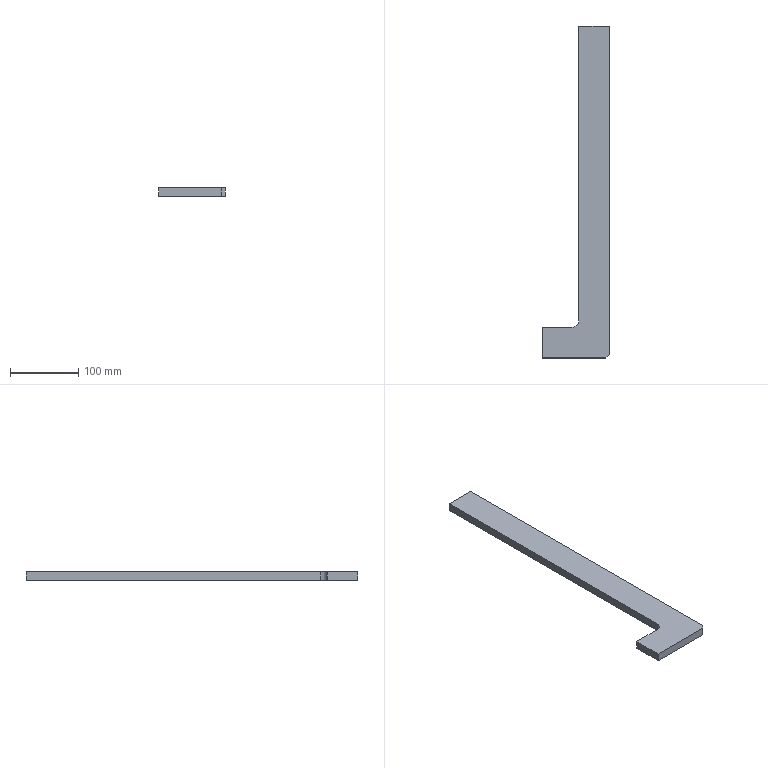Part | SolidWorks | features Chamfer 1, Extrusion 1, Fillet 1, ICE 1 | 1 solid | 10 faces | box 98 x 488 x 12 mm | volume 292248 mm3 | plane 9 | cylinder 1 | commonest cylinder face diameters 20 x1
STEP:
#1=CARTESIAN_POINT('',(49.,-239.,6.));
#2=VERTEX_POINT('',#1);
#3=CARTESIAN_POINT('',(49.,244.,6.));
#4=VERTEX_POINT('',#3);
#5=CARTESIAN_POINT('',(49.,-244.,6.));
#6=DIRECTION('',(0.,1.,0.));
#7=VECTOR('',#6,1000.);
#8=LINE('',#5,#7);
#9=EDGE_CURVE('',#2,#4,#8,.T.);
#10=ORIENTED_EDGE('',*,*,#9,.F.);
#11=CARTESIAN_POINT('',(49.,-239.,-6.));
#12=VERTEX_POINT('',#11);
#13=CARTESIAN_POINT('',(49.,-239.,6.));
#14=DIRECTION('',(0.,0.,-1.));
#15=VECTOR('',#14,1000.);
#16=LINE('',#13,#15);
#17=EDGE_CURVE('',#2,#12,#16,.T.);
#18=ORIENTED_EDGE('',*,*,#17,.T.);
#19=CARTESIAN_POINT('',(49.,244.,-6.));
#20=VERTEX_POINT('',#19);
#21=CARTESIAN_POINT('',(49.,-244.,-6.));
#22=DIRECTION('',(0.,1.,0.));
#23=VECTOR('',#22,1000.);
#24=LINE('',#21,#23);
#25=EDGE_CURVE('',#12,#20,#24,.T.);
#26=ORIENTED_EDGE('',*,*,#25,.T.);
#27=CARTESIAN_POINT('',(49.,244.,6.));
#28=DIRECTION('',(0.,0.,-1.));
#29=VECTOR('',#28,1000.);
#30=LINE('',#27,#29);
#31=EDGE_CURVE('',#4,#20,#30,.T.);
#32=ORIENTED_EDGE('',*,*,#31,.F.);
#33=EDGE_LOOP('',(#10,#18,#26,#32));
#34=FACE_OUTER_BOUND('',#33,.T.);
#35=CARTESIAN_POINT('',(49.,-244.,6.));
#36=DIRECTION('',(-1.,0.,0.));
#37=DIRECTION('',(0.,0.,1.));
#38=AXIS2_PLACEMENT_3D('',#35,#36,#37);
#39=PLANE('',#38);
#40=ADVANCED_FACE('',(#34),#39,.F.);
#41=CARTESIAN_POINT('',(4.,244.,-6.));
#42=VERTEX_POINT('',#41);
#43=CARTESIAN_POINT('',(-49.,244.,-6.));
#44=DIRECTION('',(-1.,0.,0.));
#45=VECTOR('',#44,1000.);
#46=LINE('',#43,#45);
#47=EDGE_CURVE('',#20,#42,#46,.T.);
#48=ORIENTED_EDGE('',*,*,#47,.T.);
#49=CARTESIAN_POINT('',(4.,244.,6.));
#50=VERTEX_POINT('',#49);
#51=CARTESIAN_POINT('',(4.,244.,-6.001));
#52=DIRECTION('',(0.,0.,1.));
#53=VECTOR('',#52,1000.);
#54=LINE('',#51,#53);
#55=EDGE_CURVE('',#42,#50,#54,.T.);
#56=ORIENTED_EDGE('',*,*,#55,.T.);
#57=CARTESIAN_POINT('',(-49.,244.,6.));
#58=DIRECTION('',(-1.,0.,0.));
#59=VECTOR('',#58,1000.);
#60=LINE('',#57,#59);
#61=EDGE_CURVE('',#4,#50,#60,.T.);
#62=ORIENTED_EDGE('',*,*,#61,.F.);
#63=ORIENTED_EDGE('',*,*,#31,.T.);
#64=EDGE_LOOP('',(#48,#56,#62,#63));
#65=FACE_OUTER_BOUND('',#64,.T.);
#66=CARTESIAN_POINT('',(-49.,244.,6.));
#67=DIRECTION('',(0.,-1.,0.));
#68=DIRECTION('',(0.,0.,-1.));
#69=AXIS2_PLACEMENT_3D('',#66,#67,#68);
#70=PLANE('',#69);
#71=ADVANCED_FACE('',(#65),#70,.F.);
#72=CARTESIAN_POINT('',(-49.,-199.,6.));
#73=VERTEX_POINT('',#72);
#74=CARTESIAN_POINT('',(-49.,-244.,6.));
#75=VERTEX_POINT('',#74);
#76=CARTESIAN_POINT('',(-49.,-244.,6.));
#77=DIRECTION('',(0.,-1.,0.));
#78=VECTOR('',#77,1000.);
#79=LINE('',#76,#78);
#80=EDGE_CURVE('',#73,#75,#79,.T.);
#81=ORIENTED_EDGE('',*,*,#80,.F.);
#82=CARTESIAN_POINT('',(-49.,-199.,-6.));
#83=VERTEX_POINT('',#82);
#84=CARTESIAN_POINT('',(-49.,-199.,-6.001));
#85=DIRECTION('',(0.,0.,1.));
#86=VECTOR('',#85,1000.);
#87=LINE('',#84,#86);
#88=EDGE_CURVE('',#83,#73,#87,.T.);
#89=ORIENTED_EDGE('',*,*,#88,.F.);
#90=CARTESIAN_POINT('',(-49.,-244.,-6.));
#91=VERTEX_POINT('',#90);
#92=CARTESIAN_POINT('',(-49.,-244.,-6.));
#93=DIRECTION('',(0.,-1.,0.));
#94=VECTOR('',#93,1000.);
#95=LINE('',#92,#94);
#96=EDGE_CURVE('',#83,#91,#95,.T.);
#97=ORIENTED_EDGE('',*,*,#96,.T.);
#98=CARTESIAN_POINT('',(-49.,-244.,6.));
#99=DIRECTION('',(0.,0.,-1.));
#100=VECTOR('',#99,1000.);
#101=LINE('',#98,#100);
#102=EDGE_CURVE('',#75,#91,#101,.T.);
#103=ORIENTED_EDGE('',*,*,#102,.F.);
#104=EDGE_LOOP('',(#81,#89,#97,#103));
#105=FACE_OUTER_BOUND('',#104,.T.);
#106=CARTESIAN_POINT('',(-49.,-244.,6.));
#107=DIRECTION('',(1.,0.,0.));
#108=DIRECTION('',(0.,0.,-1.));
#109=AXIS2_PLACEMENT_3D('',#106,#107,#108);
#110=PLANE('',#109);
#111=ADVANCED_FACE('',(#105),#110,.F.);
#112=CARTESIAN_POINT('',(44.,-244.,-6.));
#113=VERTEX_POINT('',#112);
#114=CARTESIAN_POINT('',(-49.,-244.,-6.));
#115=DIRECTION('',(1.,0.,0.));
#116=VECTOR('',#115,1000.);
#117=LINE('',#114,#116);
#118=EDGE_CURVE('',#91,#113,#117,.T.);
#119=ORIENTED_EDGE('',*,*,#118,.T.);
#120=CARTESIAN_POINT('',(44.,-244.,6.));
#121=VERTEX_POINT('',#120);
#122=CARTESIAN_POINT('',(44.,-244.,6.));
#123=DIRECTION('',(0.,0.,1.));
#124=VECTOR('',#123,1000.);
#125=LINE('',#122,#124);
#126=EDGE_CURVE('',#113,#121,#125,.T.);
#127=ORIENTED_EDGE('',*,*,#126,.T.);
#128=CARTESIAN_POINT('',(-49.,-244.,6.));
#129=DIRECTION('',(1.,0.,0.));
#130=VECTOR('',#129,1000.);
#131=LINE('',#128,#130);
#132=EDGE_CURVE('',#75,#121,#131,.T.);
#133=ORIENTED_EDGE('',*,*,#132,.F.);
#134=ORIENTED_EDGE('',*,*,#102,.T.);
#135=EDGE_LOOP('',(#119,#127,#133,#134));
#136=FACE_OUTER_BOUND('',#135,.T.);
#137=CARTESIAN_POINT('',(-49.,-244.,6.));
#138=DIRECTION('',(0.,1.,0.));
#139=DIRECTION('',(0.,0.,1.));
#140=AXIS2_PLACEMENT_3D('',#137,#138,#139);
#141=PLANE('',#140);
#142=ADVANCED_FACE('',(#136),#141,.F.);
#143=ORIENTED_EDGE('',*,*,#132,.T.);
#144=CARTESIAN_POINT('',(49.,-239.,6.));
#145=DIRECTION('',(0.7071,0.7071,0.));
#146=VECTOR('',#145,1000.);
#147=LINE('',#144,#146);
#148=EDGE_CURVE('',#121,#2,#147,.T.);
#149=ORIENTED_EDGE('',*,*,#148,.T.);
#150=ORIENTED_EDGE('',*,*,#9,.T.);
#151=ORIENTED_EDGE('',*,*,#61,.T.);
#152=CARTESIAN_POINT('',(4.,-189.,6.));
#153=VERTEX_POINT('',#152);
#154=CARTESIAN_POINT('',(4.,244.,6.));
#155=DIRECTION('',(0.,1.,0.));
#156=VECTOR('',#155,1000.);
#157=LINE('',#154,#156);
#158=EDGE_CURVE('',#153,#50,#157,.T.);
#159=ORIENTED_EDGE('',*,*,#158,.F.);
#160=CARTESIAN_POINT('',(-6.,-199.,6.));
#161=VERTEX_POINT('',#160);
#162=CARTESIAN_POINT('',(-6.,-189.,6.));
#163=DIRECTION('',(0.,0.,-1.));
#164=DIRECTION('',(-1.,0.,0.));
#165=AXIS2_PLACEMENT_3D('',#162,#163,#164);
#166=CIRCLE('',#165,10.);
#167=EDGE_CURVE('',#153,#161,#166,.T.);
#168=ORIENTED_EDGE('',*,*,#167,.T.);
#169=CARTESIAN_POINT('',(-49.,-199.,6.));
#170=DIRECTION('',(1.,0.,0.));
#171=VECTOR('',#170,1000.);
#172=LINE('',#169,#171);
#173=EDGE_CURVE('',#73,#161,#172,.T.);
#174=ORIENTED_EDGE('',*,*,#173,.F.);
#175=ORIENTED_EDGE('',*,*,#80,.T.);
#176=EDGE_LOOP('',(#143,#149,#150,#151,#159,#168,#174,#175));
#177=FACE_OUTER_BOUND('',#176,.T.);
#178=CARTESIAN_POINT('',(0.,0.,6.));
#179=DIRECTION('',(0.,0.,-1.));
#180=DIRECTION('',(-1.,0.,0.));
#181=AXIS2_PLACEMENT_3D('',#178,#179,#180);
#182=PLANE('',#181);
#183=ADVANCED_FACE('',(#177),#182,.F.);
#184=ORIENTED_EDGE('',*,*,#25,.F.);
#185=CARTESIAN_POINT('',(144.,-144.,-6.));
#186=DIRECTION('',(-0.7071,-0.7071,0.));
#187=VECTOR('',#186,1000.);
#188=LINE('',#185,#187);
#189=EDGE_CURVE('',#12,#113,#188,.T.);
#190=ORIENTED_EDGE('',*,*,#189,.T.);
#191=ORIENTED_EDGE('',*,*,#118,.F.);
#192=ORIENTED_EDGE('',*,*,#96,.F.);
#193=CARTESIAN_POINT('',(-6.,-199.,-6.));
#194=VERTEX_POINT('',#193);
#195=CARTESIAN_POINT('',(-49.,-199.,-6.));
#196=DIRECTION('',(1.,0.,0.));
#197=VECTOR('',#196,1000.);
#198=LINE('',#195,#197);
#199=EDGE_CURVE('',#83,#194,#198,.T.);
#200=ORIENTED_EDGE('',*,*,#199,.T.);
#201=CARTESIAN_POINT('',(4.,-189.,-6.));
#202=VERTEX_POINT('',#201);
#203=CARTESIAN_POINT('',(-6.,-189.,-6.));
#204=DIRECTION('',(0.,0.,1.));
#205=DIRECTION('',(-1.,0.,0.));
#206=AXIS2_PLACEMENT_3D('',#203,#204,#205);
#207=CIRCLE('',#206,10.);
#208=EDGE_CURVE('',#194,#202,#207,.T.);
#209=ORIENTED_EDGE('',*,*,#208,.T.);
#210=CARTESIAN_POINT('',(4.,244.,-6.));
#211=DIRECTION('',(0.,1.,0.));
#212=VECTOR('',#211,1000.);
#213=LINE('',#210,#212);
#214=EDGE_CURVE('',#202,#42,#213,.T.);
#215=ORIENTED_EDGE('',*,*,#214,.T.);
#216=ORIENTED_EDGE('',*,*,#47,.F.);
#217=EDGE_LOOP('',(#184,#190,#191,#192,#200,#209,#215,#216));
#218=FACE_OUTER_BOUND('',#217,.T.);
#219=CARTESIAN_POINT('',(0.,0.,-6.));
#220=DIRECTION('',(0.,0.,-1.));
#221=DIRECTION('',(-1.,0.,0.));
#222=AXIS2_PLACEMENT_3D('',#219,#220,#221);
#223=PLANE('',#222);
#224=ADVANCED_FACE('',(#218),#223,.T.);
#225=ORIENTED_EDGE('',*,*,#214,.F.);
#226=CARTESIAN_POINT('',(4.,-189.,6.));
#227=DIRECTION('',(0.,0.,1.));
#228=VECTOR('',#227,1000.);
#229=LINE('',#226,#228);
#230=EDGE_CURVE('',#202,#153,#229,.T.);
#231=ORIENTED_EDGE('',*,*,#230,.T.);
#232=ORIENTED_EDGE('',*,*,#158,.T.);
#233=ORIENTED_EDGE('',*,*,#55,.F.);
#234=EDGE_LOOP('',(#225,#231,#232,#233));
#235=FACE_OUTER_BOUND('',#234,.T.);
#236=CARTESIAN_POINT('',(4.,244.,-6.001));
#237=DIRECTION('',(1.,0.,0.));
#238=DIRECTION('',(0.,1.,0.));
#239=AXIS2_PLACEMENT_3D('',#236,#237,#238);
#240=PLANE('',#239);
#241=ADVANCED_FACE('',(#235),#240,.F.);
#242=ORIENTED_EDGE('',*,*,#173,.T.);
#243=CARTESIAN_POINT('',(-6.,-199.,-6.));
#244=DIRECTION('',(0.,0.,-1.));
#245=VECTOR('',#244,1000.);
#246=LINE('',#243,#245);
#247=EDGE_CURVE('',#161,#194,#246,.T.);
#248=ORIENTED_EDGE('',*,*,#247,.T.);
#249=ORIENTED_EDGE('',*,*,#199,.F.);
#250=ORIENTED_EDGE('',*,*,#88,.T.);
#251=EDGE_LOOP('',(#242,#248,#249,#250));
#252=FACE_OUTER_BOUND('',#251,.T.);
#253=CARTESIAN_POINT('',(-49.,-199.,-6.001));
#254=DIRECTION('',(0.,-1.,0.));
#255=DIRECTION('',(0.,0.,-1.));
#256=AXIS2_PLACEMENT_3D('',#253,#254,#255);
#257=PLANE('',#256);
#258=ADVANCED_FACE('',(#252),#257,.F.);
#259=ORIENTED_EDGE('',*,*,#208,.F.);
#260=ORIENTED_EDGE('',*,*,#247,.F.);
#261=ORIENTED_EDGE('',*,*,#167,.F.);
#262=ORIENTED_EDGE('',*,*,#230,.F.);
#263=EDGE_LOOP('',(#259,#260,#261,#262));
#264=FACE_OUTER_BOUND('',#263,.T.);
#265=CARTESIAN_POINT('',(-6.,-189.,-6.001));
#266=DIRECTION('',(0.,0.,-1.));
#267=DIRECTION('',(-1.,0.,0.));
#268=AXIS2_PLACEMENT_3D('',#265,#266,#267);
#269=CYLINDRICAL_SURFACE('',#268,10.);
#270=ADVANCED_FACE('',(#264),#269,.F.);
#271=ORIENTED_EDGE('',*,*,#148,.F.);
#272=ORIENTED_EDGE('',*,*,#126,.F.);
#273=ORIENTED_EDGE('',*,*,#189,.F.);
#274=ORIENTED_EDGE('',*,*,#17,.F.);
#275=EDGE_LOOP('',(#271,#272,#273,#274));
#276=FACE_OUTER_BOUND('',#275,.T.);
#277=CARTESIAN_POINT('',(49.,-239.,6.));
#278=DIRECTION('',(-0.7071,0.7071,0.));
#279=DIRECTION('',(0.,0.,-1.));
#280=AXIS2_PLACEMENT_3D('',#277,#278,#279);
#281=PLANE('',#280);
#282=ADVANCED_FACE('',(#276),#281,.F.);
#283=CLOSED_SHELL('',(#40,#71,#111,#142,#183,#224,#241,#258,#270,#282));
#284=MANIFOLD_SOLID_BREP('',#283);
#285=CARTESIAN_POINT('',(0.,0.,0.));
#286=DIRECTION('',(0.,0.,1.));
#287=DIRECTION('',(1.,0.,0.));
#288=AXIS2_PLACEMENT_3D('',#285,#286,#287);
#289=(LENGTH_UNIT()NAMED_UNIT(*)SI_UNIT(.MILLI.,.METRE.));
#290=UNCERTAINTY_MEASURE_WITH_UNIT(LENGTH_MEASURE(0.00001),#289,'','');
#291=(NAMED_UNIT(*)PLANE_ANGLE_UNIT()SI_UNIT($,.RADIAN.));
#292=(NAMED_UNIT(*)SI_UNIT($,.STERADIAN.)SOLID_ANGLE_UNIT());
#293=(GEOMETRIC_REPRESENTATION_CONTEXT(3)GLOBAL_UNCERTAINTY_ASSIGNED_CONTEXT((#290))GLOBAL_UNIT_ASSIGNED_CONTEXT((#289,#291,#292))REPRESENTATION_CONTEXT('',''));
#294=ADVANCED_BREP_SHAPE_REPRESENTATION('',(#284,#288),#293);